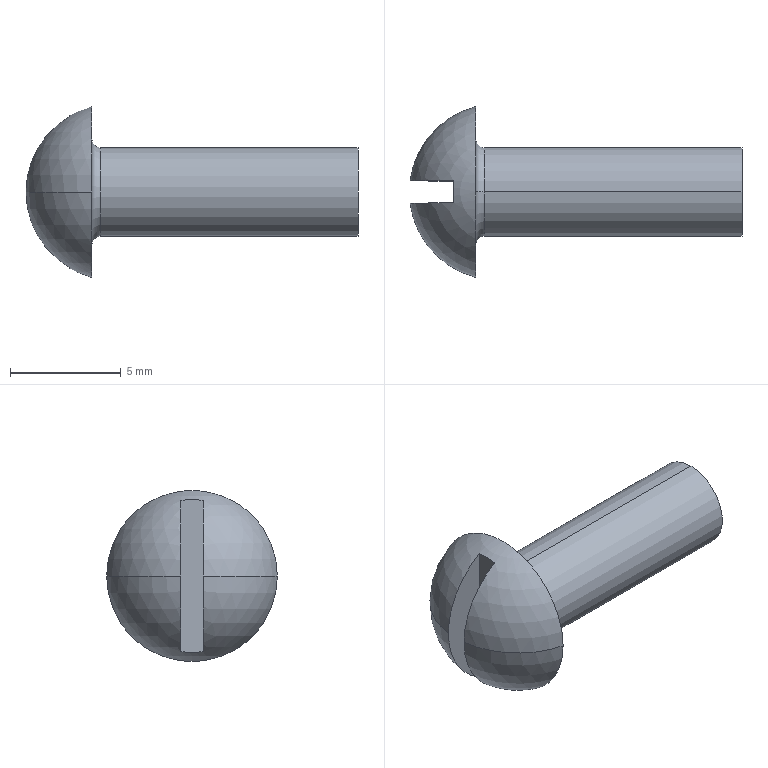Part | SolidWorks | features Cut 1, Fillet 1, Revolution 1 | 1 solid | 11 faces | box 14.968 x 7.7 x 7.7 mm | volume 225.537 mm3 | plane 5 | torus 2 | cylinder 2 | sphere 2 | commonest cylinder face diameters 4 x2
STEP:
#1=CARTESIAN_POINT('',(3.,0.,-2.4));
#2=VERTEX_POINT('',#1);
#3=CARTESIAN_POINT('',(3.,0.,2.4));
#4=VERTEX_POINT('',#3);
#5=CARTESIAN_POINT('',(3.,0.,0.));
#6=DIRECTION('',(-1.,0.,0.));
#7=DIRECTION('',(0.,0.,1.));
#8=AXIS2_PLACEMENT_3D('',#5,#6,#7);
#9=CIRCLE('',#8,2.4);
#10=EDGE_CURVE('',#2,#4,#9,.T.);
#11=ORIENTED_EDGE('',*,*,#10,.F.);
#12=CARTESIAN_POINT('',(3.4,0.,-2.));
#13=VERTEX_POINT('',#12);
#14=CARTESIAN_POINT('',(3.4,0.,-2.4));
#15=DIRECTION('',(0.,1.,0.));
#16=DIRECTION('',(0.,0.,1.));
#17=AXIS2_PLACEMENT_3D('',#14,#15,#16);
#18=CIRCLE('',#17,0.4);
#19=EDGE_CURVE('',#2,#13,#18,.T.);
#20=ORIENTED_EDGE('',*,*,#19,.T.);
#21=CARTESIAN_POINT('',(3.4,0.,2.));
#22=VERTEX_POINT('',#21);
#23=CARTESIAN_POINT('',(3.4,0.,0.));
#24=DIRECTION('',(1.,0.,0.));
#25=DIRECTION('',(0.,0.,1.));
#26=AXIS2_PLACEMENT_3D('',#23,#24,#25);
#27=CIRCLE('',#26,2.);
#28=EDGE_CURVE('',#22,#13,#27,.T.);
#29=ORIENTED_EDGE('',*,*,#28,.F.);
#30=CARTESIAN_POINT('',(3.4,0.,2.4));
#31=DIRECTION('',(0.,-1.,0.));
#32=DIRECTION('',(0.,0.,-1.));
#33=AXIS2_PLACEMENT_3D('',#30,#31,#32);
#34=CIRCLE('',#33,0.4);
#35=EDGE_CURVE('',#4,#22,#34,.T.);
#36=ORIENTED_EDGE('',*,*,#35,.F.);
#37=EDGE_LOOP('',(#11,#20,#29,#36));
#38=FACE_OUTER_BOUND('',#37,.T.);
#39=CARTESIAN_POINT('',(3.4,0.,0.));
#40=DIRECTION('',(-1.,0.,0.));
#41=DIRECTION('',(0.,0.,1.));
#42=AXIS2_PLACEMENT_3D('',#39,#40,#41);
#43=TOROIDAL_SURFACE('',#42,2.4,0.4);
#44=ADVANCED_FACE('',(#38),#43,.F.);
#45=CARTESIAN_POINT('',(15.,0.,2.));
#46=VERTEX_POINT('',#45);
#47=CARTESIAN_POINT('',(15.,0.,-2.));
#48=VERTEX_POINT('',#47);
#49=CARTESIAN_POINT('',(15.,0.,0.));
#50=DIRECTION('',(-1.,0.,0.));
#51=DIRECTION('',(0.,0.,1.));
#52=AXIS2_PLACEMENT_3D('',#49,#50,#51);
#53=CIRCLE('',#52,2.);
#54=EDGE_CURVE('',#46,#48,#53,.T.);
#55=ORIENTED_EDGE('',*,*,#54,.T.);
#56=CARTESIAN_POINT('',(0.,0.,-2.));
#57=DIRECTION('',(-1.,0.,0.));
#58=VECTOR('',#57,1000.);
#59=LINE('',#56,#58);
#60=EDGE_CURVE('',#48,#13,#59,.T.);
#61=ORIENTED_EDGE('',*,*,#60,.T.);
#62=CARTESIAN_POINT('',(3.4,0.,0.));
#63=DIRECTION('',(1.,0.,0.));
#64=DIRECTION('',(0.,0.,1.));
#65=AXIS2_PLACEMENT_3D('',#62,#63,#64);
#66=CIRCLE('',#65,2.);
#67=EDGE_CURVE('',#13,#22,#66,.T.);
#68=ORIENTED_EDGE('',*,*,#67,.T.);
#69=CARTESIAN_POINT('',(0.,0.,2.));
#70=DIRECTION('',(-1.,0.,0.));
#71=VECTOR('',#70,1000.);
#72=LINE('',#69,#71);
#73=EDGE_CURVE('',#46,#22,#72,.T.);
#74=ORIENTED_EDGE('',*,*,#73,.F.);
#75=EDGE_LOOP('',(#55,#61,#68,#74));
#76=FACE_OUTER_BOUND('',#75,.T.);
#77=CARTESIAN_POINT('',(0.,0.,0.));
#78=DIRECTION('',(-1.,0.,0.));
#79=DIRECTION('',(0.,0.,1.));
#80=AXIS2_PLACEMENT_3D('',#77,#78,#79);
#81=CYLINDRICAL_SURFACE('',#80,2.);
#82=ADVANCED_FACE('',(#76),#81,.T.);
#83=CARTESIAN_POINT('',(3.,3.85,0.));
#84=VERTEX_POINT('',#83);
#85=CARTESIAN_POINT('',(3.,-3.85,0.));
#86=VERTEX_POINT('',#85);
#87=CARTESIAN_POINT('',(3.,0.,0.));
#88=DIRECTION('',(-1.,0.,0.));
#89=DIRECTION('',(0.,0.,1.));
#90=AXIS2_PLACEMENT_3D('',#87,#88,#89);
#91=CIRCLE('',#90,3.85);
#92=EDGE_CURVE('',#84,#86,#91,.T.);
#93=ORIENTED_EDGE('',*,*,#92,.T.);
#94=CARTESIAN_POINT('',(0.03161,-0.5,0.));
#95=VERTEX_POINT('',#94);
#96=CARTESIAN_POINT('',(3.97,0.,0.));
#97=DIRECTION('',(0.,0.,-1.));
#98=DIRECTION('',(0.,1.,0.));
#99=AXIS2_PLACEMENT_3D('',#96,#97,#98);
#100=CIRCLE('',#99,3.97);
#101=EDGE_CURVE('',#86,#95,#100,.T.);
#102=ORIENTED_EDGE('',*,*,#101,.T.);
#103=CARTESIAN_POINT('',(2.,-0.5,-3.411));
#104=VERTEX_POINT('',#103);
#105=CARTESIAN_POINT('',(3.97,-0.5,0.));
#106=DIRECTION('',(0.,1.,0.));
#107=DIRECTION('',(0.,0.,1.));
#108=AXIS2_PLACEMENT_3D('',#105,#106,#107);
#109=CIRCLE('',#108,3.939);
#110=EDGE_CURVE('',#104,#95,#109,.T.);
#111=ORIENTED_EDGE('',*,*,#110,.F.);
#112=CARTESIAN_POINT('',(2.,0.5,-3.411));
#113=VERTEX_POINT('',#112);
#114=CARTESIAN_POINT('',(2.,0.,0.));
#115=DIRECTION('',(1.,0.,0.));
#116=DIRECTION('',(0.,0.,-1.));
#117=AXIS2_PLACEMENT_3D('',#114,#115,#116);
#118=CIRCLE('',#117,3.447);
#119=EDGE_CURVE('',#104,#113,#118,.T.);
#120=ORIENTED_EDGE('',*,*,#119,.T.);
#121=CARTESIAN_POINT('',(0.03161,0.5,0.));
#122=VERTEX_POINT('',#121);
#123=CARTESIAN_POINT('',(3.97,0.5,0.));
#124=DIRECTION('',(0.,-1.,0.));
#125=DIRECTION('',(0.,0.,-1.));
#126=AXIS2_PLACEMENT_3D('',#123,#124,#125);
#127=CIRCLE('',#126,3.939);
#128=EDGE_CURVE('',#122,#113,#127,.T.);
#129=ORIENTED_EDGE('',*,*,#128,.F.);
#130=CARTESIAN_POINT('',(3.97,0.,0.));
#131=DIRECTION('',(0.,0.,1.));
#132=DIRECTION('',(1.,0.,0.));
#133=AXIS2_PLACEMENT_3D('',#130,#131,#132);
#134=CIRCLE('',#133,3.97);
#135=EDGE_CURVE('',#84,#122,#134,.T.);
#136=ORIENTED_EDGE('',*,*,#135,.F.);
#137=EDGE_LOOP('',(#93,#102,#111,#120,#129,#136));
#138=FACE_OUTER_BOUND('',#137,.T.);
#139=CARTESIAN_POINT('',(3.97,0.,0.));
#140=DIRECTION('',(0.,0.,-1.));
#141=DIRECTION('',(0.,1.,0.));
#142=AXIS2_PLACEMENT_3D('',#139,#140,#141);
#143=SPHERICAL_SURFACE('',#142,3.97);
#144=ADVANCED_FACE('',(#138),#143,.T.);
#145=ORIENTED_EDGE('',*,*,#101,.F.);
#146=CARTESIAN_POINT('',(3.,0.,0.));
#147=DIRECTION('',(-1.,0.,0.));
#148=DIRECTION('',(0.,0.,1.));
#149=AXIS2_PLACEMENT_3D('',#146,#147,#148);
#150=CIRCLE('',#149,3.85);
#151=EDGE_CURVE('',#86,#84,#150,.T.);
#152=ORIENTED_EDGE('',*,*,#151,.T.);
#153=ORIENTED_EDGE('',*,*,#135,.T.);
#154=CARTESIAN_POINT('',(2.,0.5,3.411));
#155=VERTEX_POINT('',#154);
#156=CARTESIAN_POINT('',(3.97,0.5,0.));
#157=DIRECTION('',(0.,-1.,0.));
#158=DIRECTION('',(0.,0.,-1.));
#159=AXIS2_PLACEMENT_3D('',#156,#157,#158);
#160=CIRCLE('',#159,3.939);
#161=EDGE_CURVE('',#155,#122,#160,.T.);
#162=ORIENTED_EDGE('',*,*,#161,.F.);
#163=CARTESIAN_POINT('',(2.,-0.5,3.411));
#164=VERTEX_POINT('',#163);
#165=CARTESIAN_POINT('',(2.,0.,0.));
#166=DIRECTION('',(1.,0.,0.));
#167=DIRECTION('',(0.,0.,-1.));
#168=AXIS2_PLACEMENT_3D('',#165,#166,#167);
#169=CIRCLE('',#168,3.447);
#170=EDGE_CURVE('',#155,#164,#169,.T.);
#171=ORIENTED_EDGE('',*,*,#170,.T.);
#172=CARTESIAN_POINT('',(3.97,-0.5,0.));
#173=DIRECTION('',(0.,1.,0.));
#174=DIRECTION('',(0.,0.,1.));
#175=AXIS2_PLACEMENT_3D('',#172,#173,#174);
#176=CIRCLE('',#175,3.939);
#177=EDGE_CURVE('',#95,#164,#176,.T.);
#178=ORIENTED_EDGE('',*,*,#177,.F.);
#179=EDGE_LOOP('',(#145,#152,#153,#162,#171,#178));
#180=FACE_OUTER_BOUND('',#179,.T.);
#181=CARTESIAN_POINT('',(3.97,0.,0.));
#182=DIRECTION('',(0.,0.,-1.));
#183=DIRECTION('',(0.,1.,0.));
#184=AXIS2_PLACEMENT_3D('',#181,#182,#183);
#185=SPHERICAL_SURFACE('',#184,3.97);
#186=ADVANCED_FACE('',(#180),#185,.T.);
#187=CARTESIAN_POINT('',(3.,0.,0.));
#188=DIRECTION('',(-1.,0.,0.));
#189=DIRECTION('',(0.,0.,1.));
#190=AXIS2_PLACEMENT_3D('',#187,#188,#189);
#191=CIRCLE('',#190,2.4);
#192=EDGE_CURVE('',#4,#2,#191,.T.);
#193=ORIENTED_EDGE('',*,*,#192,.T.);
#194=ORIENTED_EDGE('',*,*,#10,.T.);
#195=EDGE_LOOP('',(#193,#194));
#196=FACE_BOUND('',#195,.T.);
#197=ORIENTED_EDGE('',*,*,#92,.F.);
#198=ORIENTED_EDGE('',*,*,#151,.F.);
#199=EDGE_LOOP('',(#197,#198));
#200=FACE_OUTER_BOUND('',#199,.T.);
#201=CARTESIAN_POINT('',(3.,3.85,0.));
#202=DIRECTION('',(-1.,0.,0.));
#203=DIRECTION('',(0.,0.,1.));
#204=AXIS2_PLACEMENT_3D('',#201,#202,#203);
#205=PLANE('',#204);
#206=ADVANCED_FACE('',(#196,#200),#205,.F.);
#207=ORIENTED_EDGE('',*,*,#60,.F.);
#208=CARTESIAN_POINT('',(15.,0.,0.));
#209=DIRECTION('',(-1.,0.,0.));
#210=DIRECTION('',(0.,0.,1.));
#211=AXIS2_PLACEMENT_3D('',#208,#209,#210);
#212=CIRCLE('',#211,2.);
#213=EDGE_CURVE('',#48,#46,#212,.T.);
#214=ORIENTED_EDGE('',*,*,#213,.T.);
#215=ORIENTED_EDGE('',*,*,#73,.T.);
#216=ORIENTED_EDGE('',*,*,#28,.T.);
#217=EDGE_LOOP('',(#207,#214,#215,#216));
#218=FACE_OUTER_BOUND('',#217,.T.);
#219=CARTESIAN_POINT('',(0.,0.,0.));
#220=DIRECTION('',(-1.,0.,0.));
#221=DIRECTION('',(0.,0.,1.));
#222=AXIS2_PLACEMENT_3D('',#219,#220,#221);
#223=CYLINDRICAL_SURFACE('',#222,2.);
#224=ADVANCED_FACE('',(#218),#223,.T.);
#225=ORIENTED_EDGE('',*,*,#54,.F.);
#226=ORIENTED_EDGE('',*,*,#213,.F.);
#227=EDGE_LOOP('',(#225,#226));
#228=FACE_OUTER_BOUND('',#227,.T.);
#229=CARTESIAN_POINT('',(15.,2.,0.));
#230=DIRECTION('',(-1.,0.,0.));
#231=DIRECTION('',(0.,0.,1.));
#232=AXIS2_PLACEMENT_3D('',#229,#230,#231);
#233=PLANE('',#232);
#234=ADVANCED_FACE('',(#228),#233,.F.);
#235=ORIENTED_EDGE('',*,*,#161,.T.);
#236=ORIENTED_EDGE('',*,*,#128,.T.);
#237=CARTESIAN_POINT('',(2.,0.5,-3.85));
#238=DIRECTION('',(0.,0.,1.));
#239=VECTOR('',#238,1000.);
#240=LINE('',#237,#239);
#241=EDGE_CURVE('',#113,#155,#240,.T.);
#242=ORIENTED_EDGE('',*,*,#241,.T.);
#243=EDGE_LOOP('',(#235,#236,#242));
#244=FACE_OUTER_BOUND('',#243,.T.);
#245=CARTESIAN_POINT('',(2.,0.5,-3.85));
#246=DIRECTION('',(0.,-1.,0.));
#247=DIRECTION('',(0.,0.,-1.));
#248=AXIS2_PLACEMENT_3D('',#245,#246,#247);
#249=PLANE('',#248);
#250=ADVANCED_FACE('',(#244),#249,.T.);
#251=ORIENTED_EDGE('',*,*,#110,.T.);
#252=ORIENTED_EDGE('',*,*,#177,.T.);
#253=CARTESIAN_POINT('',(2.,-0.5,3.85));
#254=DIRECTION('',(0.,0.,-1.));
#255=VECTOR('',#254,1000.);
#256=LINE('',#253,#255);
#257=EDGE_CURVE('',#164,#104,#256,.T.);
#258=ORIENTED_EDGE('',*,*,#257,.T.);
#259=EDGE_LOOP('',(#251,#252,#258));
#260=FACE_OUTER_BOUND('',#259,.T.);
#261=CARTESIAN_POINT('',(2.,-0.5,3.85));
#262=DIRECTION('',(0.,1.,0.));
#263=DIRECTION('',(0.,0.,1.));
#264=AXIS2_PLACEMENT_3D('',#261,#262,#263);
#265=PLANE('',#264);
#266=ADVANCED_FACE('',(#260),#265,.T.);
#267=ORIENTED_EDGE('',*,*,#241,.F.);
#268=ORIENTED_EDGE('',*,*,#119,.F.);
#269=ORIENTED_EDGE('',*,*,#257,.F.);
#270=ORIENTED_EDGE('',*,*,#170,.F.);
#271=EDGE_LOOP('',(#267,#268,#269,#270));
#272=FACE_OUTER_BOUND('',#271,.T.);
#273=CARTESIAN_POINT('',(2.,0.5,-3.85));
#274=DIRECTION('',(1.,0.,0.));
#275=DIRECTION('',(0.,0.,-1.));
#276=AXIS2_PLACEMENT_3D('',#273,#274,#275);
#277=PLANE('',#276);
#278=ADVANCED_FACE('',(#272),#277,.F.);
#279=ORIENTED_EDGE('',*,*,#19,.F.);
#280=ORIENTED_EDGE('',*,*,#192,.F.);
#281=ORIENTED_EDGE('',*,*,#35,.T.);
#282=ORIENTED_EDGE('',*,*,#67,.F.);
#283=EDGE_LOOP('',(#279,#280,#281,#282));
#284=FACE_OUTER_BOUND('',#283,.T.);
#285=CARTESIAN_POINT('',(3.4,0.,0.));
#286=DIRECTION('',(-1.,0.,0.));
#287=DIRECTION('',(0.,0.,1.));
#288=AXIS2_PLACEMENT_3D('',#285,#286,#287);
#289=TOROIDAL_SURFACE('',#288,2.4,0.4);
#290=ADVANCED_FACE('',(#284),#289,.F.);
#291=CLOSED_SHELL('',(#44,#82,#144,#186,#206,#224,#234,#250,#266,#278,#290));
#292=MANIFOLD_SOLID_BREP('',#291);
#293=CARTESIAN_POINT('',(0.,0.,0.));
#294=DIRECTION('',(0.,0.,1.));
#295=DIRECTION('',(1.,0.,0.));
#296=AXIS2_PLACEMENT_3D('',#293,#294,#295);
#297=(LENGTH_UNIT()NAMED_UNIT(*)SI_UNIT(.MILLI.,.METRE.));
#298=UNCERTAINTY_MEASURE_WITH_UNIT(LENGTH_MEASURE(0.00001),#297,'','');
#299=(NAMED_UNIT(*)PLANE_ANGLE_UNIT()SI_UNIT($,.RADIAN.));
#300=(NAMED_UNIT(*)SI_UNIT($,.STERADIAN.)SOLID_ANGLE_UNIT());
#301=(GEOMETRIC_REPRESENTATION_CONTEXT(3)GLOBAL_UNCERTAINTY_ASSIGNED_CONTEXT((#298))GLOBAL_UNIT_ASSIGNED_CONTEXT((#297,#299,#300))REPRESENTATION_CONTEXT('',''));
#302=ADVANCED_BREP_SHAPE_REPRESENTATION('',(#292,#296),#301);